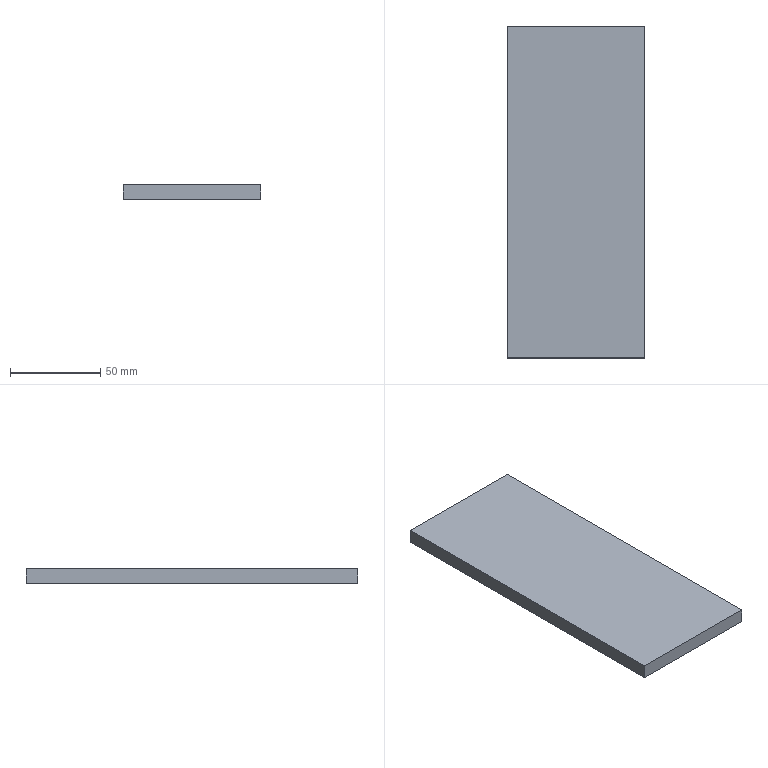Part | SolidWorks | features Extrusion 1 | 1 solid | 6 faces | box 76.2 x 184.2 x 8 mm | volume 112288 mm3 | plane 6
STEP:
#1=CARTESIAN_POINT('',(-38.1,92.1,-4.));
#2=VERTEX_POINT('',#1);
#3=CARTESIAN_POINT('',(-38.1,-92.1,-4.));
#4=VERTEX_POINT('',#3);
#5=CARTESIAN_POINT('',(-38.1,92.1,-4.));
#6=DIRECTION('',(0.,-1.,0.));
#7=VECTOR('',#6,1000.);
#8=LINE('',#5,#7);
#9=EDGE_CURVE('',#2,#4,#8,.T.);
#10=ORIENTED_EDGE('',*,*,#9,.T.);
#11=CARTESIAN_POINT('',(-38.1,-92.1,4.));
#12=VERTEX_POINT('',#11);
#13=CARTESIAN_POINT('',(-38.1,-92.1,4.));
#14=DIRECTION('',(0.,0.,-1.));
#15=VECTOR('',#14,1000.);
#16=LINE('',#13,#15);
#17=EDGE_CURVE('',#12,#4,#16,.T.);
#18=ORIENTED_EDGE('',*,*,#17,.F.);
#19=CARTESIAN_POINT('',(-38.1,92.1,4.));
#20=VERTEX_POINT('',#19);
#21=CARTESIAN_POINT('',(-38.1,92.1,4.));
#22=DIRECTION('',(0.,-1.,0.));
#23=VECTOR('',#22,1000.);
#24=LINE('',#21,#23);
#25=EDGE_CURVE('',#20,#12,#24,.T.);
#26=ORIENTED_EDGE('',*,*,#25,.F.);
#27=CARTESIAN_POINT('',(-38.1,92.1,4.));
#28=DIRECTION('',(0.,0.,-1.));
#29=VECTOR('',#28,1000.);
#30=LINE('',#27,#29);
#31=EDGE_CURVE('',#20,#2,#30,.T.);
#32=ORIENTED_EDGE('',*,*,#31,.T.);
#33=EDGE_LOOP('',(#10,#18,#26,#32));
#34=FACE_OUTER_BOUND('',#33,.T.);
#35=CARTESIAN_POINT('',(-38.1,92.1,4.));
#36=DIRECTION('',(1.,0.,0.));
#37=DIRECTION('',(0.,1.,0.));
#38=AXIS2_PLACEMENT_3D('',#35,#36,#37);
#39=PLANE('',#38);
#40=ADVANCED_FACE('',(#34),#39,.F.);
#41=CARTESIAN_POINT('',(38.1,-92.1,-4.));
#42=VERTEX_POINT('',#41);
#43=CARTESIAN_POINT('',(-38.1,-92.1,-4.));
#44=DIRECTION('',(1.,0.,0.));
#45=VECTOR('',#44,1000.);
#46=LINE('',#43,#45);
#47=EDGE_CURVE('',#4,#42,#46,.T.);
#48=ORIENTED_EDGE('',*,*,#47,.T.);
#49=CARTESIAN_POINT('',(38.1,-92.1,4.));
#50=VERTEX_POINT('',#49);
#51=CARTESIAN_POINT('',(38.1,-92.1,4.));
#52=DIRECTION('',(0.,0.,-1.));
#53=VECTOR('',#52,1000.);
#54=LINE('',#51,#53);
#55=EDGE_CURVE('',#50,#42,#54,.T.);
#56=ORIENTED_EDGE('',*,*,#55,.F.);
#57=CARTESIAN_POINT('',(-38.1,-92.1,4.));
#58=DIRECTION('',(1.,0.,0.));
#59=VECTOR('',#58,1000.);
#60=LINE('',#57,#59);
#61=EDGE_CURVE('',#12,#50,#60,.T.);
#62=ORIENTED_EDGE('',*,*,#61,.F.);
#63=ORIENTED_EDGE('',*,*,#17,.T.);
#64=EDGE_LOOP('',(#48,#56,#62,#63));
#65=FACE_OUTER_BOUND('',#64,.T.);
#66=CARTESIAN_POINT('',(-38.1,-92.1,4.));
#67=DIRECTION('',(0.,1.,0.));
#68=DIRECTION('',(-1.,0.,0.));
#69=AXIS2_PLACEMENT_3D('',#66,#67,#68);
#70=PLANE('',#69);
#71=ADVANCED_FACE('',(#65),#70,.F.);
#72=CARTESIAN_POINT('',(38.1,92.1,-4.));
#73=VERTEX_POINT('',#72);
#74=CARTESIAN_POINT('',(38.1,92.1,-4.));
#75=DIRECTION('',(0.,1.,0.));
#76=VECTOR('',#75,1000.);
#77=LINE('',#74,#76);
#78=EDGE_CURVE('',#42,#73,#77,.T.);
#79=ORIENTED_EDGE('',*,*,#78,.T.);
#80=CARTESIAN_POINT('',(38.1,92.1,4.));
#81=VERTEX_POINT('',#80);
#82=CARTESIAN_POINT('',(38.1,92.1,4.));
#83=DIRECTION('',(0.,0.,-1.));
#84=VECTOR('',#83,1000.);
#85=LINE('',#82,#84);
#86=EDGE_CURVE('',#81,#73,#85,.T.);
#87=ORIENTED_EDGE('',*,*,#86,.F.);
#88=CARTESIAN_POINT('',(38.1,92.1,4.));
#89=DIRECTION('',(0.,1.,0.));
#90=VECTOR('',#89,1000.);
#91=LINE('',#88,#90);
#92=EDGE_CURVE('',#50,#81,#91,.T.);
#93=ORIENTED_EDGE('',*,*,#92,.F.);
#94=ORIENTED_EDGE('',*,*,#55,.T.);
#95=EDGE_LOOP('',(#79,#87,#93,#94));
#96=FACE_OUTER_BOUND('',#95,.T.);
#97=CARTESIAN_POINT('',(38.1,92.1,4.));
#98=DIRECTION('',(-1.,0.,0.));
#99=DIRECTION('',(0.,-1.,0.));
#100=AXIS2_PLACEMENT_3D('',#97,#98,#99);
#101=PLANE('',#100);
#102=ADVANCED_FACE('',(#96),#101,.F.);
#103=CARTESIAN_POINT('',(-38.1,92.1,-4.));
#104=DIRECTION('',(-1.,0.,0.));
#105=VECTOR('',#104,1000.);
#106=LINE('',#103,#105);
#107=EDGE_CURVE('',#73,#2,#106,.T.);
#108=ORIENTED_EDGE('',*,*,#107,.T.);
#109=ORIENTED_EDGE('',*,*,#31,.F.);
#110=CARTESIAN_POINT('',(-38.1,92.1,4.));
#111=DIRECTION('',(-1.,0.,0.));
#112=VECTOR('',#111,1000.);
#113=LINE('',#110,#112);
#114=EDGE_CURVE('',#81,#20,#113,.T.);
#115=ORIENTED_EDGE('',*,*,#114,.F.);
#116=ORIENTED_EDGE('',*,*,#86,.T.);
#117=EDGE_LOOP('',(#108,#109,#115,#116));
#118=FACE_OUTER_BOUND('',#117,.T.);
#119=CARTESIAN_POINT('',(-38.1,92.1,4.));
#120=DIRECTION('',(0.,-1.,0.));
#121=DIRECTION('',(1.,0.,0.));
#122=AXIS2_PLACEMENT_3D('',#119,#120,#121);
#123=PLANE('',#122);
#124=ADVANCED_FACE('',(#118),#123,.F.);
#125=ORIENTED_EDGE('',*,*,#25,.T.);
#126=ORIENTED_EDGE('',*,*,#61,.T.);
#127=ORIENTED_EDGE('',*,*,#92,.T.);
#128=ORIENTED_EDGE('',*,*,#114,.T.);
#129=EDGE_LOOP('',(#125,#126,#127,#128));
#130=FACE_OUTER_BOUND('',#129,.T.);
#131=CARTESIAN_POINT('',(0.,0.,4.));
#132=DIRECTION('',(0.,0.,1.));
#133=DIRECTION('',(1.,0.,0.));
#134=AXIS2_PLACEMENT_3D('',#131,#132,#133);
#135=PLANE('',#134);
#136=ADVANCED_FACE('',(#130),#135,.T.);
#137=ORIENTED_EDGE('',*,*,#9,.F.);
#138=ORIENTED_EDGE('',*,*,#107,.F.);
#139=ORIENTED_EDGE('',*,*,#78,.F.);
#140=ORIENTED_EDGE('',*,*,#47,.F.);
#141=EDGE_LOOP('',(#137,#138,#139,#140));
#142=FACE_OUTER_BOUND('',#141,.T.);
#143=CARTESIAN_POINT('',(0.,0.,-4.));
#144=DIRECTION('',(0.,0.,1.));
#145=DIRECTION('',(1.,0.,0.));
#146=AXIS2_PLACEMENT_3D('',#143,#144,#145);
#147=PLANE('',#146);
#148=ADVANCED_FACE('',(#142),#147,.F.);
#149=CLOSED_SHELL('',(#40,#71,#102,#124,#136,#148));
#150=MANIFOLD_SOLID_BREP('',#149);
#151=CARTESIAN_POINT('',(0.,0.,0.));
#152=DIRECTION('',(0.,0.,1.));
#153=DIRECTION('',(1.,0.,0.));
#154=AXIS2_PLACEMENT_3D('',#151,#152,#153);
#155=(LENGTH_UNIT()NAMED_UNIT(*)SI_UNIT(.MILLI.,.METRE.));
#156=UNCERTAINTY_MEASURE_WITH_UNIT(LENGTH_MEASURE(0.00001),#155,'','');
#157=(NAMED_UNIT(*)PLANE_ANGLE_UNIT()SI_UNIT($,.RADIAN.));
#158=(NAMED_UNIT(*)SI_UNIT($,.STERADIAN.)SOLID_ANGLE_UNIT());
#159=(GEOMETRIC_REPRESENTATION_CONTEXT(3)GLOBAL_UNCERTAINTY_ASSIGNED_CONTEXT((#156))GLOBAL_UNIT_ASSIGNED_CONTEXT((#155,#157,#158))REPRESENTATION_CONTEXT('',''));
#160=ADVANCED_BREP_SHAPE_REPRESENTATION('',(#150,#154),#159);